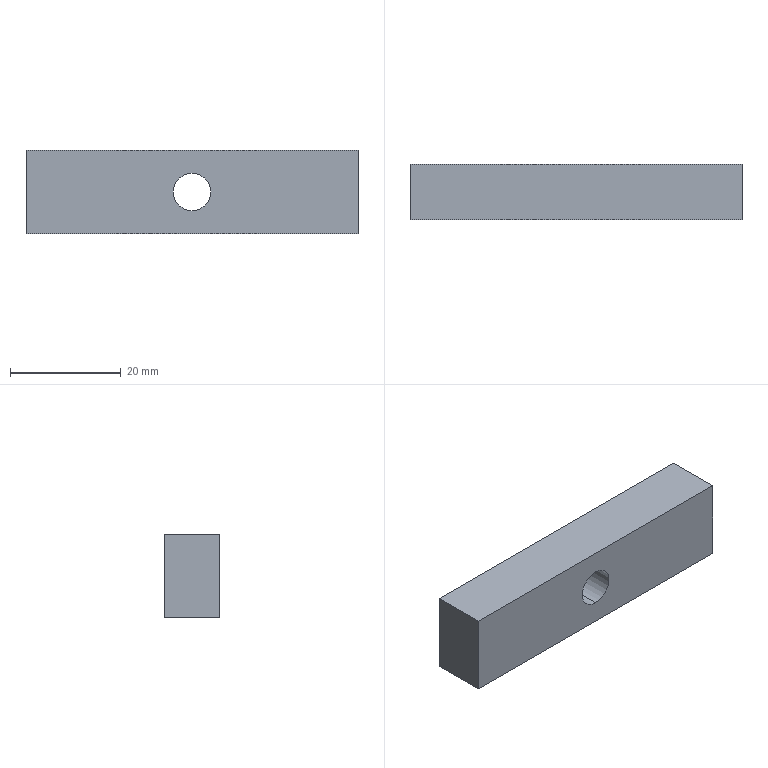Part | STEP file | PN_0036_plate_default_machined_ | 1 solid | 8 faces | box 60 x 10 x 15 mm | volume 8637 mm3 | plane 6 | cylinder 2 | commonest cylinder face diameters 6.8 x2
STEP:
#1=CARTESIAN_POINT('',(0.,0.,0.));
#2=DIRECTION('',(0.,0.,1.));
#3=DIRECTION('',(1.,0.,0.));
#4=AXIS2_PLACEMENT_3D('',#1,#2,#3);
#5=CARTESIAN_POINT('',(30.,-10.,-4.1));
#6=VERTEX_POINT('',#5);
#7=CARTESIAN_POINT('',(30.,0.,-4.1));
#8=VERTEX_POINT('',#7);
#9=CARTESIAN_POINT('',(30.,0.,-4.1));
#10=DIRECTION('',(0.,1.,0.));
#11=VECTOR('',#10,1.);
#12=LINE('',#9,#11);
#13=CARTESIAN_POINT('',(30.,0.,-7.5));
#14=DIRECTION('',(0.,1.,0.));
#15=DIRECTION('',(0.,0.,1.));
#16=AXIS2_PLACEMENT_3D('',#13,#14,#15);
#17=CYLINDRICAL_SURFACE('',#16,3.4);
#18=CARTESIAN_POINT('',(6.283,0.));
#19=DIRECTION('',(0.,1.));
#20=VECTOR('',#19,1.);
#21=LINE('',#18,#20);
#22=(GEOMETRIC_REPRESENTATION_CONTEXT(2)PARAMETRIC_REPRESENTATION_CONTEXT()REPRESENTATION_CONTEXT('',''));
#23=DEFINITIONAL_REPRESENTATION('',(#21),#22);
#24=PCURVE('',#17,#23);
#25=CARTESIAN_POINT('',(30.,0.,-7.5));
#26=DIRECTION('',(0.,1.,0.));
#27=DIRECTION('',(0.,0.,1.));
#28=AXIS2_PLACEMENT_3D('',#25,#26,#27);
#29=CYLINDRICAL_SURFACE('',#28,3.4);
#30=CARTESIAN_POINT('',(0.,0.));
#31=DIRECTION('',(0.,1.));
#32=VECTOR('',#31,1.);
#33=LINE('',#30,#32);
#34=(GEOMETRIC_REPRESENTATION_CONTEXT(2)PARAMETRIC_REPRESENTATION_CONTEXT()REPRESENTATION_CONTEXT('',''));
#35=DEFINITIONAL_REPRESENTATION('',(#33),#34);
#36=PCURVE('',#29,#35);
#37=SURFACE_CURVE('',#12,(#24,#36),.PCURVE_S1.);
#38=EDGE_CURVE('',#6,#8,#37,.T.);
#39=ORIENTED_EDGE('',*,*,#38,.T.);
#40=CARTESIAN_POINT('',(30.,0.,-10.9));
#41=VERTEX_POINT('',#40);
#42=CARTESIAN_POINT('',(30.,0.,-7.5));
#43=DIRECTION('',(0.,-1.,0.));
#44=DIRECTION('',(0.,0.,1.));
#45=AXIS2_PLACEMENT_3D('',#42,#43,#44);
#46=CIRCLE('',#45,3.4);
#47=CARTESIAN_POINT('',(6.283,0.));
#48=DIRECTION('',(-1.,0.));
#49=VECTOR('',#48,1.);
#50=LINE('',#47,#49);
#51=(GEOMETRIC_REPRESENTATION_CONTEXT(2)PARAMETRIC_REPRESENTATION_CONTEXT()REPRESENTATION_CONTEXT('',''));
#52=DEFINITIONAL_REPRESENTATION('',(#50),#51);
#53=PCURVE('',#17,#52);
#54=CARTESIAN_POINT('',(0.,0.,0.));
#55=DIRECTION('',(0.,-1.,0.));
#56=DIRECTION('',(0.,0.,-1.));
#57=AXIS2_PLACEMENT_3D('',#54,#55,#56);
#58=PLANE('',#57);
#59=CARTESIAN_POINT('',(7.5,30.));
#60=DIRECTION('',(-1.,0.));
#61=AXIS2_PLACEMENT_2D('',#59,#60);
#62=CIRCLE('',#61,3.4);
#63=(GEOMETRIC_REPRESENTATION_CONTEXT(2)PARAMETRIC_REPRESENTATION_CONTEXT()REPRESENTATION_CONTEXT('',''));
#64=DEFINITIONAL_REPRESENTATION('',(#62),#63);
#65=PCURVE('',#58,#64);
#66=SURFACE_CURVE('',#46,(#53,#65),.PCURVE_S1.);
#67=EDGE_CURVE('',#8,#41,#66,.T.);
#68=ORIENTED_EDGE('',*,*,#67,.T.);
#69=CARTESIAN_POINT('',(30.,-10.,-10.9));
#70=VERTEX_POINT('',#69);
#71=CARTESIAN_POINT('',(30.,0.,-10.9));
#72=DIRECTION('',(0.,1.,0.));
#73=VECTOR('',#72,1.);
#74=LINE('',#71,#73);
#75=CARTESIAN_POINT('',(3.142,0.));
#76=DIRECTION('',(0.,1.));
#77=VECTOR('',#76,1.);
#78=LINE('',#75,#77);
#79=(GEOMETRIC_REPRESENTATION_CONTEXT(2)PARAMETRIC_REPRESENTATION_CONTEXT()REPRESENTATION_CONTEXT('',''));
#80=DEFINITIONAL_REPRESENTATION('',(#78),#79);
#81=PCURVE('',#17,#80);
#82=CARTESIAN_POINT('',(3.142,0.));
#83=DIRECTION('',(0.,1.));
#84=VECTOR('',#83,1.);
#85=LINE('',#82,#84);
#86=(GEOMETRIC_REPRESENTATION_CONTEXT(2)PARAMETRIC_REPRESENTATION_CONTEXT()REPRESENTATION_CONTEXT('',''));
#87=DEFINITIONAL_REPRESENTATION('',(#85),#86);
#88=PCURVE('',#29,#87);
#89=SURFACE_CURVE('',#74,(#81,#88),.PCURVE_S1.);
#90=EDGE_CURVE('',#70,#41,#89,.T.);
#91=ORIENTED_EDGE('',*,*,#90,.F.);
#92=CARTESIAN_POINT('',(30.,-10.,-7.5));
#93=DIRECTION('',(0.,1.,0.));
#94=DIRECTION('',(0.,0.,1.));
#95=AXIS2_PLACEMENT_3D('',#92,#93,#94);
#96=CIRCLE('',#95,3.4);
#97=CARTESIAN_POINT('',(0.,-10.));
#98=DIRECTION('',(1.,0.));
#99=VECTOR('',#98,1.);
#100=LINE('',#97,#99);
#101=(GEOMETRIC_REPRESENTATION_CONTEXT(2)PARAMETRIC_REPRESENTATION_CONTEXT()REPRESENTATION_CONTEXT('',''));
#102=DEFINITIONAL_REPRESENTATION('',(#100),#101);
#103=PCURVE('',#17,#102);
#104=CARTESIAN_POINT('',(0.,-10.,0.));
#105=DIRECTION('',(0.,-1.,0.));
#106=DIRECTION('',(0.,0.,-1.));
#107=AXIS2_PLACEMENT_3D('',#104,#105,#106);
#108=PLANE('',#107);
#109=CARTESIAN_POINT('',(4.1,30.));
#110=CARTESIAN_POINT('',(4.1,35.889));
#111=CARTESIAN_POINT('',(9.2,32.944));
#112=CARTESIAN_POINT('',(14.3,30.));
#113=CARTESIAN_POINT('',(9.2,27.056));
#114=CARTESIAN_POINT('',(4.1,24.111));
#115=CARTESIAN_POINT('',(4.1,30.));
#116=(BOUNDED_CURVE()B_SPLINE_CURVE(2,(#109,#110,#111,#112,#113,#114,#115),.UNSPECIFIED.,.T.,.F.)B_SPLINE_CURVE_WITH_KNOTS((1,2,2,2,2,1),(-2.094,0.,2.094,4.189,6.283,8.378),.UNSPECIFIED.)CURVE()GEOMETRIC_REPRESENTATION_ITEM()RATIONAL_B_SPLINE_CURVE((1.,0.5,1.,0.5,1.,0.5,1.))REPRESENTATION_ITEM(''));
#117=(GEOMETRIC_REPRESENTATION_CONTEXT(2)PARAMETRIC_REPRESENTATION_CONTEXT()REPRESENTATION_CONTEXT('',''));
#118=DEFINITIONAL_REPRESENTATION('',(#116),#117);
#119=PCURVE('',#108,#118);
#120=SURFACE_CURVE('',#96,(#103,#119),.PCURVE_S1.);
#121=EDGE_CURVE('',#70,#6,#120,.T.);
#122=ORIENTED_EDGE('',*,*,#121,.T.);
#123=EDGE_LOOP('',(#39,#68,#91,#122));
#124=FACE_BOUND('',#123,.F.);
#125=ADVANCED_FACE('',(#124),#17,.F.);
#126=CARTESIAN_POINT('',(60.,-10.,-15.));
#127=VERTEX_POINT('',#126);
#128=CARTESIAN_POINT('',(60.,-10.,0.));
#129=VERTEX_POINT('',#128);
#130=CARTESIAN_POINT('',(60.,-10.,0.));
#131=DIRECTION('',(0.,0.,1.));
#132=VECTOR('',#131,1.);
#133=LINE('',#130,#132);
#134=CARTESIAN_POINT('',(0.,60.));
#135=DIRECTION('',(-1.,0.));
#136=VECTOR('',#135,1.);
#137=LINE('',#134,#136);
#138=(GEOMETRIC_REPRESENTATION_CONTEXT(2)PARAMETRIC_REPRESENTATION_CONTEXT()REPRESENTATION_CONTEXT('',''));
#139=DEFINITIONAL_REPRESENTATION('',(#137),#138);
#140=PCURVE('',#108,#139);
#141=CARTESIAN_POINT('',(60.,-10.,0.));
#142=DIRECTION('',(1.,0.,0.));
#143=DIRECTION('',(0.,0.,-1.));
#144=AXIS2_PLACEMENT_3D('',#141,#142,#143);
#145=PLANE('',#144);
#146=CARTESIAN_POINT('',(0.,0.));
#147=DIRECTION('',(-1.,0.));
#148=VECTOR('',#147,1.);
#149=LINE('',#146,#148);
#150=(GEOMETRIC_REPRESENTATION_CONTEXT(2)PARAMETRIC_REPRESENTATION_CONTEXT()REPRESENTATION_CONTEXT('',''));
#151=DEFINITIONAL_REPRESENTATION('',(#149),#150);
#152=PCURVE('',#145,#151);
#153=SURFACE_CURVE('',#133,(#140,#152),.PCURVE_S1.);
#154=EDGE_CURVE('',#127,#129,#153,.T.);
#155=ORIENTED_EDGE('',*,*,#154,.T.);
#156=CARTESIAN_POINT('',(0.,-10.,0.));
#157=VERTEX_POINT('',#156);
#158=CARTESIAN_POINT('',(0.,-10.,0.));
#159=DIRECTION('',(-1.,0.,0.));
#160=VECTOR('',#159,1.);
#161=LINE('',#158,#160);
#162=CARTESIAN_POINT('',(0.,0.));
#163=DIRECTION('',(0.,-1.));
#164=VECTOR('',#163,1.);
#165=LINE('',#162,#164);
#166=(GEOMETRIC_REPRESENTATION_CONTEXT(2)PARAMETRIC_REPRESENTATION_CONTEXT()REPRESENTATION_CONTEXT('',''));
#167=DEFINITIONAL_REPRESENTATION('',(#165),#166);
#168=PCURVE('',#108,#167);
#169=CARTESIAN_POINT('',(0.,-10.,0.));
#170=DIRECTION('',(0.,0.,1.));
#171=DIRECTION('',(1.,0.,0.));
#172=AXIS2_PLACEMENT_3D('',#169,#170,#171);
#173=PLANE('',#172);
#174=CARTESIAN_POINT('',(0.,0.));
#175=DIRECTION('',(-1.,0.));
#176=VECTOR('',#175,1.);
#177=LINE('',#174,#176);
#178=(GEOMETRIC_REPRESENTATION_CONTEXT(2)PARAMETRIC_REPRESENTATION_CONTEXT()REPRESENTATION_CONTEXT('',''));
#179=DEFINITIONAL_REPRESENTATION('',(#177),#178);
#180=PCURVE('',#173,#179);
#181=SURFACE_CURVE('',#161,(#168,#180),.PCURVE_S1.);
#182=EDGE_CURVE('',#129,#157,#181,.T.);
#183=ORIENTED_EDGE('',*,*,#182,.T.);
#184=CARTESIAN_POINT('',(0.,-10.,-15.));
#185=VERTEX_POINT('',#184);
#186=CARTESIAN_POINT('',(0.,-10.,0.));
#187=DIRECTION('',(0.,0.,-1.));
#188=VECTOR('',#187,1.);
#189=LINE('',#186,#188);
#190=CARTESIAN_POINT('',(0.,0.));
#191=DIRECTION('',(1.,0.));
#192=VECTOR('',#191,1.);
#193=LINE('',#190,#192);
#194=(GEOMETRIC_REPRESENTATION_CONTEXT(2)PARAMETRIC_REPRESENTATION_CONTEXT()REPRESENTATION_CONTEXT('',''));
#195=DEFINITIONAL_REPRESENTATION('',(#193),#194);
#196=PCURVE('',#108,#195);
#197=CARTESIAN_POINT('',(0.,-10.,0.));
#198=DIRECTION('',(-1.,0.,0.));
#199=DIRECTION('',(0.,0.,1.));
#200=AXIS2_PLACEMENT_3D('',#197,#198,#199);
#201=PLANE('',#200);
#202=CARTESIAN_POINT('',(0.,0.));
#203=DIRECTION('',(-1.,0.));
#204=VECTOR('',#203,1.);
#205=LINE('',#202,#204);
#206=(GEOMETRIC_REPRESENTATION_CONTEXT(2)PARAMETRIC_REPRESENTATION_CONTEXT()REPRESENTATION_CONTEXT('',''));
#207=DEFINITIONAL_REPRESENTATION('',(#205),#206);
#208=PCURVE('',#201,#207);
#209=SURFACE_CURVE('',#189,(#196,#208),.PCURVE_S1.);
#210=EDGE_CURVE('',#157,#185,#209,.T.);
#211=ORIENTED_EDGE('',*,*,#210,.T.);
#212=CARTESIAN_POINT('',(0.,-10.,-15.));
#213=DIRECTION('',(1.,0.,0.));
#214=VECTOR('',#213,1.);
#215=LINE('',#212,#214);
#216=CARTESIAN_POINT('',(15.,0.));
#217=DIRECTION('',(0.,1.));
#218=VECTOR('',#217,1.);
#219=LINE('',#216,#218);
#220=(GEOMETRIC_REPRESENTATION_CONTEXT(2)PARAMETRIC_REPRESENTATION_CONTEXT()REPRESENTATION_CONTEXT('',''));
#221=DEFINITIONAL_REPRESENTATION('',(#219),#220);
#222=PCURVE('',#108,#221);
#223=CARTESIAN_POINT('',(0.,-10.,-15.));
#224=DIRECTION('',(0.,0.,-1.));
#225=DIRECTION('',(-1.,0.,0.));
#226=AXIS2_PLACEMENT_3D('',#223,#224,#225);
#227=PLANE('',#226);
#228=CARTESIAN_POINT('',(0.,0.));
#229=DIRECTION('',(-1.,0.));
#230=VECTOR('',#229,1.);
#231=LINE('',#228,#230);
#232=(GEOMETRIC_REPRESENTATION_CONTEXT(2)PARAMETRIC_REPRESENTATION_CONTEXT()REPRESENTATION_CONTEXT('',''));
#233=DEFINITIONAL_REPRESENTATION('',(#231),#232);
#234=PCURVE('',#227,#233);
#235=SURFACE_CURVE('',#215,(#222,#234),.PCURVE_S1.);
#236=EDGE_CURVE('',#185,#127,#235,.T.);
#237=ORIENTED_EDGE('',*,*,#236,.T.);
#238=EDGE_LOOP('',(#155,#183,#211,#237));
#239=FACE_BOUND('',#238,.T.);
#240=CARTESIAN_POINT('',(30.,-10.,-7.5));
#241=DIRECTION('',(0.,1.,0.));
#242=DIRECTION('',(0.,0.,1.));
#243=AXIS2_PLACEMENT_3D('',#240,#241,#242);
#244=CIRCLE('',#243,3.4);
#245=CARTESIAN_POINT('',(4.1,30.));
#246=CARTESIAN_POINT('',(4.1,35.889));
#247=CARTESIAN_POINT('',(9.2,32.944));
#248=CARTESIAN_POINT('',(14.3,30.));
#249=CARTESIAN_POINT('',(9.2,27.056));
#250=CARTESIAN_POINT('',(4.1,24.111));
#251=CARTESIAN_POINT('',(4.1,30.));
#252=(BOUNDED_CURVE()B_SPLINE_CURVE(2,(#245,#246,#247,#248,#249,#250,#251),.UNSPECIFIED.,.T.,.F.)B_SPLINE_CURVE_WITH_KNOTS((1,2,2,2,2,1),(-2.094,0.,2.094,4.189,6.283,8.378),.UNSPECIFIED.)CURVE()GEOMETRIC_REPRESENTATION_ITEM()RATIONAL_B_SPLINE_CURVE((1.,0.5,1.,0.5,1.,0.5,1.))REPRESENTATION_ITEM(''));
#253=(GEOMETRIC_REPRESENTATION_CONTEXT(2)PARAMETRIC_REPRESENTATION_CONTEXT()REPRESENTATION_CONTEXT('',''));
#254=DEFINITIONAL_REPRESENTATION('',(#252),#253);
#255=PCURVE('',#108,#254);
#256=CARTESIAN_POINT('',(0.,-10.));
#257=DIRECTION('',(1.,0.));
#258=VECTOR('',#257,1.);
#259=LINE('',#256,#258);
#260=(GEOMETRIC_REPRESENTATION_CONTEXT(2)PARAMETRIC_REPRESENTATION_CONTEXT()REPRESENTATION_CONTEXT('',''));
#261=DEFINITIONAL_REPRESENTATION('',(#259),#260);
#262=PCURVE('',#29,#261);
#263=SURFACE_CURVE('',#244,(#255,#262),.PCURVE_S1.);
#264=EDGE_CURVE('',#6,#70,#263,.T.);
#265=ORIENTED_EDGE('',*,*,#264,.T.);
#266=ORIENTED_EDGE('',*,*,#121,.T.);
#267=EDGE_LOOP('',(#265,#266));
#268=FACE_BOUND('',#267,.T.);
#269=ADVANCED_FACE('',(#239,#268),#108,.T.);
#270=ORIENTED_EDGE('',*,*,#182,.F.);
#271=CARTESIAN_POINT('',(60.,0.,0.));
#272=VERTEX_POINT('',#271);
#273=CARTESIAN_POINT('',(60.,-10.,0.));
#274=DIRECTION('',(0.,1.,0.));
#275=VECTOR('',#274,1.);
#276=LINE('',#273,#275);
#277=CARTESIAN_POINT('',(60.,0.));
#278=DIRECTION('',(0.,1.));
#279=VECTOR('',#278,1.);
#280=LINE('',#277,#279);
#281=(GEOMETRIC_REPRESENTATION_CONTEXT(2)PARAMETRIC_REPRESENTATION_CONTEXT()REPRESENTATION_CONTEXT('',''));
#282=DEFINITIONAL_REPRESENTATION('',(#280),#281);
#283=PCURVE('',#173,#282);
#284=CARTESIAN_POINT('',(0.,0.));
#285=DIRECTION('',(0.,1.));
#286=VECTOR('',#285,1.);
#287=LINE('',#284,#286);
#288=(GEOMETRIC_REPRESENTATION_CONTEXT(2)PARAMETRIC_REPRESENTATION_CONTEXT()REPRESENTATION_CONTEXT('',''));
#289=DEFINITIONAL_REPRESENTATION('',(#287),#288);
#290=PCURVE('',#145,#289);
#291=SURFACE_CURVE('',#276,(#283,#290),.PCURVE_S1.);
#292=EDGE_CURVE('',#129,#272,#291,.T.);
#293=ORIENTED_EDGE('',*,*,#292,.T.);
#294=CARTESIAN_POINT('',(0.,0.,0.));
#295=VERTEX_POINT('',#294);
#296=CARTESIAN_POINT('',(0.,0.,0.));
#297=DIRECTION('',(-1.,0.,0.));
#298=VECTOR('',#297,1.);
#299=LINE('',#296,#298);
#300=CARTESIAN_POINT('',(0.,10.));
#301=DIRECTION('',(-1.,0.));
#302=VECTOR('',#301,1.);
#303=LINE('',#300,#302);
#304=(GEOMETRIC_REPRESENTATION_CONTEXT(2)PARAMETRIC_REPRESENTATION_CONTEXT()REPRESENTATION_CONTEXT('',''));
#305=DEFINITIONAL_REPRESENTATION('',(#303),#304);
#306=PCURVE('',#173,#305);
#307=CARTESIAN_POINT('',(0.,0.));
#308=DIRECTION('',(0.,-1.));
#309=VECTOR('',#308,1.);
#310=LINE('',#307,#309);
#311=(GEOMETRIC_REPRESENTATION_CONTEXT(2)PARAMETRIC_REPRESENTATION_CONTEXT()REPRESENTATION_CONTEXT('',''));
#312=DEFINITIONAL_REPRESENTATION('',(#310),#311);
#313=PCURVE('',#58,#312);
#314=SURFACE_CURVE('',#299,(#306,#313),.PCURVE_S1.);
#315=EDGE_CURVE('',#272,#295,#314,.T.);
#316=ORIENTED_EDGE('',*,*,#315,.T.);
#317=CARTESIAN_POINT('',(0.,-10.,0.));
#318=DIRECTION('',(0.,-1.,0.));
#319=VECTOR('',#318,1.);
#320=LINE('',#317,#319);
#321=CARTESIAN_POINT('',(0.,0.));
#322=DIRECTION('',(0.,-1.));
#323=VECTOR('',#322,1.);
#324=LINE('',#321,#323);
#325=(GEOMETRIC_REPRESENTATION_CONTEXT(2)PARAMETRIC_REPRESENTATION_CONTEXT()REPRESENTATION_CONTEXT('',''));
#326=DEFINITIONAL_REPRESENTATION('',(#324),#325);
#327=PCURVE('',#173,#326);
#328=CARTESIAN_POINT('',(0.,0.));
#329=DIRECTION('',(0.,-1.));
#330=VECTOR('',#329,1.);
#331=LINE('',#328,#330);
#332=(GEOMETRIC_REPRESENTATION_CONTEXT(2)PARAMETRIC_REPRESENTATION_CONTEXT()REPRESENTATION_CONTEXT('',''));
#333=DEFINITIONAL_REPRESENTATION('',(#331),#332);
#334=PCURVE('',#201,#333);
#335=SURFACE_CURVE('',#320,(#327,#334),.PCURVE_S1.);
#336=EDGE_CURVE('',#295,#157,#335,.T.);
#337=ORIENTED_EDGE('',*,*,#336,.T.);
#338=EDGE_LOOP('',(#270,#293,#316,#337));
#339=FACE_BOUND('',#338,.T.);
#340=ADVANCED_FACE('',(#339),#173,.T.);
#341=ORIENTED_EDGE('',*,*,#154,.F.);
#342=CARTESIAN_POINT('',(60.,0.,-15.));
#343=VERTEX_POINT('',#342);
#344=CARTESIAN_POINT('',(60.,-10.,-15.));
#345=DIRECTION('',(0.,1.,0.));
#346=VECTOR('',#345,1.);
#347=LINE('',#344,#346);
#348=CARTESIAN_POINT('',(15.,0.));
#349=DIRECTION('',(0.,1.));
#350=VECTOR('',#349,1.);
#351=LINE('',#348,#350);
#352=(GEOMETRIC_REPRESENTATION_CONTEXT(2)PARAMETRIC_REPRESENTATION_CONTEXT()REPRESENTATION_CONTEXT('',''));
#353=DEFINITIONAL_REPRESENTATION('',(#351),#352);
#354=PCURVE('',#145,#353);
#355=CARTESIAN_POINT('',(-60.,0.));
#356=DIRECTION('',(0.,1.));
#357=VECTOR('',#356,1.);
#358=LINE('',#355,#357);
#359=(GEOMETRIC_REPRESENTATION_CONTEXT(2)PARAMETRIC_REPRESENTATION_CONTEXT()REPRESENTATION_CONTEXT('',''));
#360=DEFINITIONAL_REPRESENTATION('',(#358),#359);
#361=PCURVE('',#227,#360);
#362=SURFACE_CURVE('',#347,(#354,#361),.PCURVE_S1.);
#363=EDGE_CURVE('',#127,#343,#362,.T.);
#364=ORIENTED_EDGE('',*,*,#363,.T.);
#365=CARTESIAN_POINT('',(60.,0.,0.));
#366=DIRECTION('',(0.,0.,1.));
#367=VECTOR('',#366,1.);
#368=LINE('',#365,#367);
#369=CARTESIAN_POINT('',(0.,10.));
#370=DIRECTION('',(-1.,0.));
#371=VECTOR('',#370,1.);
#372=LINE('',#369,#371);
#373=(GEOMETRIC_REPRESENTATION_CONTEXT(2)PARAMETRIC_REPRESENTATION_CONTEXT()REPRESENTATION_CONTEXT('',''));
#374=DEFINITIONAL_REPRESENTATION('',(#372),#373);
#375=PCURVE('',#145,#374);
#376=CARTESIAN_POINT('',(0.,60.));
#377=DIRECTION('',(-1.,0.));
#378=VECTOR('',#377,1.);
#379=LINE('',#376,#378);
#380=(GEOMETRIC_REPRESENTATION_CONTEXT(2)PARAMETRIC_REPRESENTATION_CONTEXT()REPRESENTATION_CONTEXT('',''));
#381=DEFINITIONAL_REPRESENTATION('',(#379),#380);
#382=PCURVE('',#58,#381);
#383=SURFACE_CURVE('',#368,(#375,#382),.PCURVE_S1.);
#384=EDGE_CURVE('',#343,#272,#383,.T.);
#385=ORIENTED_EDGE('',*,*,#384,.T.);
#386=ORIENTED_EDGE('',*,*,#292,.F.);
#387=EDGE_LOOP('',(#341,#364,#385,#386));
#388=FACE_BOUND('',#387,.T.);
#389=ADVANCED_FACE('',(#388),#145,.T.);
#390=ORIENTED_EDGE('',*,*,#236,.F.);
#391=CARTESIAN_POINT('',(0.,0.,-15.));
#392=VERTEX_POINT('',#391);
#393=CARTESIAN_POINT('',(0.,-10.,-15.));
#394=DIRECTION('',(0.,1.,0.));
#395=VECTOR('',#394,1.);
#396=LINE('',#393,#395);
#397=CARTESIAN_POINT('',(0.,0.));
#398=DIRECTION('',(0.,1.));
#399=VECTOR('',#398,1.);
#400=LINE('',#397,#399);
#401=(GEOMETRIC_REPRESENTATION_CONTEXT(2)PARAMETRIC_REPRESENTATION_CONTEXT()REPRESENTATION_CONTEXT('',''));
#402=DEFINITIONAL_REPRESENTATION('',(#400),#401);
#403=PCURVE('',#227,#402);
#404=CARTESIAN_POINT('',(-15.,0.));
#405=DIRECTION('',(0.,1.));
#406=VECTOR('',#405,1.);
#407=LINE('',#404,#406);
#408=(GEOMETRIC_REPRESENTATION_CONTEXT(2)PARAMETRIC_REPRESENTATION_CONTEXT()REPRESENTATION_CONTEXT('',''));
#409=DEFINITIONAL_REPRESENTATION('',(#407),#408);
#410=PCURVE('',#201,#409);
#411=SURFACE_CURVE('',#396,(#403,#410),.PCURVE_S1.);
#412=EDGE_CURVE('',#185,#392,#411,.T.);
#413=ORIENTED_EDGE('',*,*,#412,.T.);
#414=CARTESIAN_POINT('',(0.,0.,-15.));
#415=DIRECTION('',(1.,0.,0.));
#416=VECTOR('',#415,1.);
#417=LINE('',#414,#416);
#418=CARTESIAN_POINT('',(0.,10.));
#419=DIRECTION('',(-1.,0.));
#420=VECTOR('',#419,1.);
#421=LINE('',#418,#420);
#422=(GEOMETRIC_REPRESENTATION_CONTEXT(2)PARAMETRIC_REPRESENTATION_CONTEXT()REPRESENTATION_CONTEXT('',''));
#423=DEFINITIONAL_REPRESENTATION('',(#421),#422);
#424=PCURVE('',#227,#423);
#425=CARTESIAN_POINT('',(15.,0.));
#426=DIRECTION('',(0.,1.));
#427=VECTOR('',#426,1.);
#428=LINE('',#425,#427);
#429=(GEOMETRIC_REPRESENTATION_CONTEXT(2)PARAMETRIC_REPRESENTATION_CONTEXT()REPRESENTATION_CONTEXT('',''));
#430=DEFINITIONAL_REPRESENTATION('',(#428),#429);
#431=PCURVE('',#58,#430);
#432=SURFACE_CURVE('',#417,(#424,#431),.PCURVE_S1.);
#433=EDGE_CURVE('',#392,#343,#432,.T.);
#434=ORIENTED_EDGE('',*,*,#433,.T.);
#435=ORIENTED_EDGE('',*,*,#363,.F.);
#436=EDGE_LOOP('',(#390,#413,#434,#435));
#437=FACE_BOUND('',#436,.T.);
#438=ADVANCED_FACE('',(#437),#227,.T.);
#439=ORIENTED_EDGE('',*,*,#210,.F.);
#440=ORIENTED_EDGE('',*,*,#336,.F.);
#441=CARTESIAN_POINT('',(0.,0.,0.));
#442=DIRECTION('',(0.,0.,-1.));
#443=VECTOR('',#442,1.);
#444=LINE('',#441,#443);
#445=CARTESIAN_POINT('',(0.,10.));
#446=DIRECTION('',(-1.,0.));
#447=VECTOR('',#446,1.);
#448=LINE('',#445,#447);
#449=(GEOMETRIC_REPRESENTATION_CONTEXT(2)PARAMETRIC_REPRESENTATION_CONTEXT()REPRESENTATION_CONTEXT('',''));
#450=DEFINITIONAL_REPRESENTATION('',(#448),#449);
#451=PCURVE('',#201,#450);
#452=CARTESIAN_POINT('',(0.,0.));
#453=DIRECTION('',(1.,0.));
#454=VECTOR('',#453,1.);
#455=LINE('',#452,#454);
#456=(GEOMETRIC_REPRESENTATION_CONTEXT(2)PARAMETRIC_REPRESENTATION_CONTEXT()REPRESENTATION_CONTEXT('',''));
#457=DEFINITIONAL_REPRESENTATION('',(#455),#456);
#458=PCURVE('',#58,#457);
#459=SURFACE_CURVE('',#444,(#451,#458),.PCURVE_S1.);
#460=EDGE_CURVE('',#295,#392,#459,.T.);
#461=ORIENTED_EDGE('',*,*,#460,.T.);
#462=ORIENTED_EDGE('',*,*,#412,.F.);
#463=EDGE_LOOP('',(#439,#440,#461,#462));
#464=FACE_BOUND('',#463,.T.);
#465=ADVANCED_FACE('',(#464),#201,.T.);
#466=CARTESIAN_POINT('',(30.,0.,-7.5));
#467=DIRECTION('',(0.,-1.,0.));
#468=DIRECTION('',(0.,0.,1.));
#469=AXIS2_PLACEMENT_3D('',#466,#467,#468);
#470=CIRCLE('',#469,3.4);
#471=CARTESIAN_POINT('',(6.283,0.));
#472=DIRECTION('',(-1.,0.));
#473=VECTOR('',#472,1.);
#474=LINE('',#471,#473);
#475=(GEOMETRIC_REPRESENTATION_CONTEXT(2)PARAMETRIC_REPRESENTATION_CONTEXT()REPRESENTATION_CONTEXT('',''));
#476=DEFINITIONAL_REPRESENTATION('',(#474),#475);
#477=PCURVE('',#29,#476);
#478=CARTESIAN_POINT('',(7.5,30.));
#479=DIRECTION('',(-1.,0.));
#480=AXIS2_PLACEMENT_2D('',#478,#479);
#481=CIRCLE('',#480,3.4);
#482=(GEOMETRIC_REPRESENTATION_CONTEXT(2)PARAMETRIC_REPRESENTATION_CONTEXT()REPRESENTATION_CONTEXT('',''));
#483=DEFINITIONAL_REPRESENTATION('',(#481),#482);
#484=PCURVE('',#58,#483);
#485=SURFACE_CURVE('',#470,(#477,#484),.PCURVE_S1.);
#486=EDGE_CURVE('',#41,#8,#485,.T.);
#487=ORIENTED_EDGE('',*,*,#486,.T.);
#488=ORIENTED_EDGE('',*,*,#38,.F.);
#489=ORIENTED_EDGE('',*,*,#264,.T.);
#490=ORIENTED_EDGE('',*,*,#90,.T.);
#491=EDGE_LOOP('',(#487,#488,#489,#490));
#492=FACE_BOUND('',#491,.F.);
#493=ADVANCED_FACE('',(#492),#29,.F.);
#494=ORIENTED_EDGE('',*,*,#315,.F.);
#495=ORIENTED_EDGE('',*,*,#384,.F.);
#496=ORIENTED_EDGE('',*,*,#433,.F.);
#497=ORIENTED_EDGE('',*,*,#460,.F.);
#498=EDGE_LOOP('',(#494,#495,#496,#497));
#499=FACE_BOUND('',#498,.T.);
#500=ORIENTED_EDGE('',*,*,#67,.T.);
#501=ORIENTED_EDGE('',*,*,#486,.T.);
#502=EDGE_LOOP('',(#500,#501));
#503=FACE_BOUND('',#502,.T.);
#504=ADVANCED_FACE('',(#499,#503),#58,.F.);
#505=CLOSED_SHELL('',(#125,#269,#340,#389,#438,#465,#493,#504));
#506=MANIFOLD_SOLID_BREP('',#505);
#507=(LENGTH_UNIT()NAMED_UNIT(*)SI_UNIT(.MILLI.,.METRE.));
#508=UNCERTAINTY_MEASURE_WITH_UNIT(LENGTH_MEASURE(0.0000001),#507,'','');
#509=(NAMED_UNIT(*)PLANE_ANGLE_UNIT()SI_UNIT($,.RADIAN.));
#510=(NAMED_UNIT(*)SI_UNIT($,.STERADIAN.)SOLID_ANGLE_UNIT());
#511=(GEOMETRIC_REPRESENTATION_CONTEXT(3)GLOBAL_UNCERTAINTY_ASSIGNED_CONTEXT((#508))GLOBAL_UNIT_ASSIGNED_CONTEXT((#507,#509,#510))REPRESENTATION_CONTEXT('',''));
#512=ADVANCED_BREP_SHAPE_REPRESENTATION('',(#4,#506),#511);